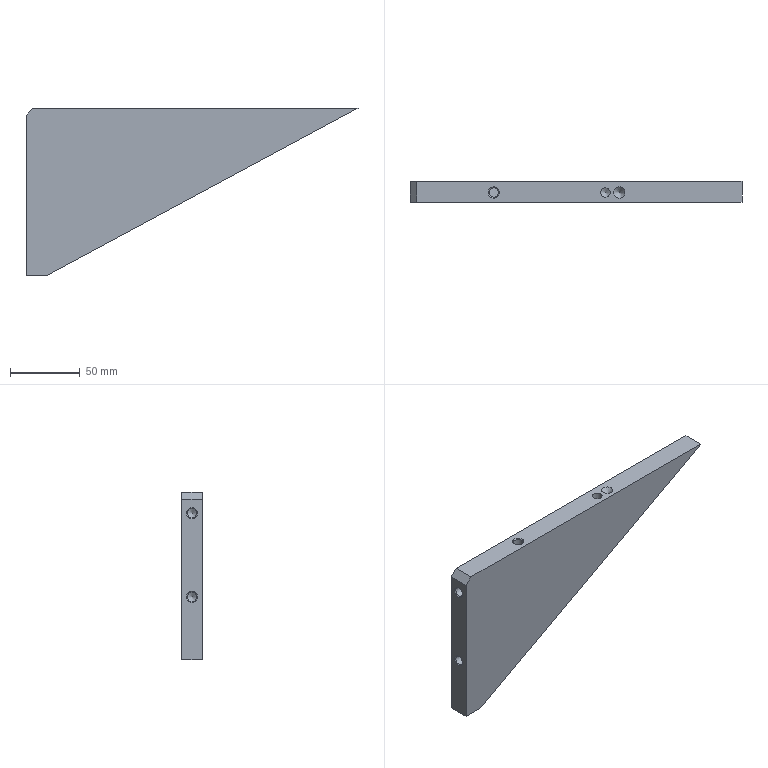Part | STEP file | 冲床-300配套压波_id978_x_t | 1 solid | 19 faces | box 237.857 x 15 x 120 mm | volume 223740 mm3 | cone 8 | plane 7 | cylinder 4 | commonest cylinder face diameters 6.8 x4
STEP:
#1=CARTESIAN_POINT('',(1960.,75.,-230.));
#2=VERTEX_POINT('',#1);
#3=CARTESIAN_POINT('',(2192.857,75.,-230.));
#4=VERTEX_POINT('',#3);
#5=CARTESIAN_POINT('',(2165.,75.,-230.));
#6=DIRECTION('',(1.,0.,0.));
#7=VECTOR('',#6,1.);
#8=LINE('',#5,#7);
#9=EDGE_CURVE('',#2,#4,#8,.T.);
#10=ORIENTED_EDGE('',*,*,#9,.F.);
#11=CARTESIAN_POINT('',(1955.,75.,-235.));
#12=VERTEX_POINT('',#11);
#13=CARTESIAN_POINT('',(1967.5,75.,-222.5));
#14=DIRECTION('',(-0.7071,0.,-0.7071));
#15=VECTOR('',#14,1.);
#16=LINE('',#13,#15);
#17=EDGE_CURVE('',#2,#12,#16,.T.);
#18=ORIENTED_EDGE('',*,*,#17,.T.);
#19=CARTESIAN_POINT('',(1955.,75.,-350.));
#20=VERTEX_POINT('',#19);
#21=CARTESIAN_POINT('',(1955.,75.,-230.));
#22=DIRECTION('',(0.,0.,1.));
#23=VECTOR('',#22,1.);
#24=LINE('',#21,#23);
#25=EDGE_CURVE('',#20,#12,#24,.T.);
#26=ORIENTED_EDGE('',*,*,#25,.F.);
#27=CARTESIAN_POINT('',(1970.,75.,-350.));
#28=VERTEX_POINT('',#27);
#29=CARTESIAN_POINT('',(1955.,75.,-350.));
#30=DIRECTION('',(-1.,0.,0.));
#31=VECTOR('',#30,1.);
#32=LINE('',#29,#31);
#33=EDGE_CURVE('',#28,#20,#32,.T.);
#34=ORIENTED_EDGE('',*,*,#33,.F.);
#35=CARTESIAN_POINT('',(1970.,75.,-350.));
#36=DIRECTION('',(-0.8805,0.,-0.4741));
#37=VECTOR('',#36,1.);
#38=LINE('',#35,#37);
#39=EDGE_CURVE('',#4,#28,#38,.T.);
#40=ORIENTED_EDGE('',*,*,#39,.F.);
#41=EDGE_LOOP('',(#10,#18,#26,#34,#40));
#42=FACE_OUTER_BOUND('',#41,.T.);
#43=CARTESIAN_POINT('',(2135.,75.,-390.));
#44=DIRECTION('',(0.,1.,0.));
#45=DIRECTION('',(0.,0.,-1.));
#46=AXIS2_PLACEMENT_3D('',#43,#44,#45);
#47=PLANE('',#46);
#48=ADVANCED_FACE('',(#42),#47,.F.);
#49=CARTESIAN_POINT('',(1955.,90.,-350.));
#50=VERTEX_POINT('',#49);
#51=CARTESIAN_POINT('',(1955.,-58.5,-350.));
#52=DIRECTION('',(0.,-1.,0.));
#53=VECTOR('',#52,1.);
#54=LINE('',#51,#53);
#55=EDGE_CURVE('',#50,#20,#54,.T.);
#56=ORIENTED_EDGE('',*,*,#55,.F.);
#57=CARTESIAN_POINT('',(1970.,90.,-350.));
#58=VERTEX_POINT('',#57);
#59=CARTESIAN_POINT('',(1955.,90.,-350.));
#60=DIRECTION('',(-1.,0.,0.));
#61=VECTOR('',#60,1.);
#62=LINE('',#59,#61);
#63=EDGE_CURVE('',#58,#50,#62,.T.);
#64=ORIENTED_EDGE('',*,*,#63,.F.);
#65=CARTESIAN_POINT('',(1970.,-58.5,-350.));
#66=DIRECTION('',(0.,-1.,0.));
#67=VECTOR('',#66,1.);
#68=LINE('',#65,#67);
#69=EDGE_CURVE('',#58,#28,#68,.T.);
#70=ORIENTED_EDGE('',*,*,#69,.T.);
#71=ORIENTED_EDGE('',*,*,#33,.T.);
#72=EDGE_LOOP('',(#56,#64,#70,#71));
#73=FACE_OUTER_BOUND('',#72,.T.);
#74=CARTESIAN_POINT('',(1955.,-58.5,-350.));
#75=DIRECTION('',(0.,0.,-1.));
#76=DIRECTION('',(-1.,0.,0.));
#77=AXIS2_PLACEMENT_3D('',#74,#75,#76);
#78=PLANE('',#77);
#79=ADVANCED_FACE('',(#73),#78,.T.);
#80=ORIENTED_EDGE('',*,*,#69,.F.);
#81=CARTESIAN_POINT('',(2192.857,90.,-230.));
#82=VERTEX_POINT('',#81);
#83=CARTESIAN_POINT('',(1970.,90.,-350.));
#84=DIRECTION('',(-0.8805,0.,-0.4741));
#85=VECTOR('',#84,1.);
#86=LINE('',#83,#85);
#87=EDGE_CURVE('',#82,#58,#86,.T.);
#88=ORIENTED_EDGE('',*,*,#87,.F.);
#89=CARTESIAN_POINT('',(2192.857,-58.5,-230.));
#90=DIRECTION('',(0.,1.,0.));
#91=VECTOR('',#90,1.);
#92=LINE('',#89,#91);
#93=EDGE_CURVE('',#4,#82,#92,.T.);
#94=ORIENTED_EDGE('',*,*,#93,.F.);
#95=ORIENTED_EDGE('',*,*,#39,.T.);
#96=EDGE_LOOP('',(#80,#88,#94,#95));
#97=FACE_OUTER_BOUND('',#96,.T.);
#98=CARTESIAN_POINT('',(1970.,-58.5,-350.));
#99=DIRECTION('',(0.4741,0.,-0.8805));
#100=DIRECTION('',(-0.8805,0.,-0.4741));
#101=AXIS2_PLACEMENT_3D('',#98,#99,#100);
#102=PLANE('',#101);
#103=ADVANCED_FACE('',(#97),#102,.T.);
#104=CARTESIAN_POINT('',(1955.,90.,-235.));
#105=VERTEX_POINT('',#104);
#106=CARTESIAN_POINT('',(1955.,90.,-230.));
#107=DIRECTION('',(0.,0.,1.));
#108=VECTOR('',#107,1.);
#109=LINE('',#106,#108);
#110=EDGE_CURVE('',#50,#105,#109,.T.);
#111=ORIENTED_EDGE('',*,*,#110,.T.);
#112=CARTESIAN_POINT('',(1960.,90.,-230.));
#113=VERTEX_POINT('',#112);
#114=CARTESIAN_POINT('',(1960.,90.,-230.));
#115=DIRECTION('',(0.7071,0.,0.7071));
#116=VECTOR('',#115,1.);
#117=LINE('',#114,#116);
#118=EDGE_CURVE('',#105,#113,#117,.T.);
#119=ORIENTED_EDGE('',*,*,#118,.T.);
#120=CARTESIAN_POINT('',(2165.,90.,-230.));
#121=DIRECTION('',(1.,0.,0.));
#122=VECTOR('',#121,1.);
#123=LINE('',#120,#122);
#124=EDGE_CURVE('',#113,#82,#123,.T.);
#125=ORIENTED_EDGE('',*,*,#124,.T.);
#126=ORIENTED_EDGE('',*,*,#87,.T.);
#127=ORIENTED_EDGE('',*,*,#63,.T.);
#128=EDGE_LOOP('',(#111,#119,#125,#126,#127));
#129=FACE_OUTER_BOUND('',#128,.T.);
#130=CARTESIAN_POINT('',(1455.,90.,-90.));
#131=DIRECTION('',(0.,-1.,0.));
#132=DIRECTION('',(0.,0.,1.));
#133=AXIS2_PLACEMENT_3D('',#130,#131,#132);
#134=PLANE('',#133);
#135=ADVANCED_FACE('',(#129),#134,.F.);
#136=CARTESIAN_POINT('',(1955.,82.5,-301.));
#137=VERTEX_POINT('',#136);
#138=CARTESIAN_POINT('',(1955.,82.5,-305.));
#139=DIRECTION('',(1.,0.,0.));
#140=DIRECTION('',(0.,0.,1.));
#141=AXIS2_PLACEMENT_3D('',#138,#139,#140);
#142=CIRCLE('',#141,4.);
#143=EDGE_CURVE('',#137,#137,#142,.T.);
#144=ORIENTED_EDGE('',*,*,#143,.T.);
#145=EDGE_LOOP('',(#144));
#146=FACE_BOUND('',#145,.T.);
#147=CARTESIAN_POINT('',(1955.,82.5,-241.));
#148=VERTEX_POINT('',#147);
#149=CARTESIAN_POINT('',(1955.,82.5,-245.));
#150=DIRECTION('',(1.,0.,0.));
#151=DIRECTION('',(0.,0.,1.));
#152=AXIS2_PLACEMENT_3D('',#149,#150,#151);
#153=CIRCLE('',#152,4.);
#154=EDGE_CURVE('',#148,#148,#153,.T.);
#155=ORIENTED_EDGE('',*,*,#154,.T.);
#156=EDGE_LOOP('',(#155));
#157=FACE_BOUND('',#156,.T.);
#158=ORIENTED_EDGE('',*,*,#25,.T.);
#159=CARTESIAN_POINT('',(1955.,-58.5,-235.));
#160=DIRECTION('',(0.,1.,0.));
#161=VECTOR('',#160,1.);
#162=LINE('',#159,#161);
#163=EDGE_CURVE('',#12,#105,#162,.T.);
#164=ORIENTED_EDGE('',*,*,#163,.T.);
#165=ORIENTED_EDGE('',*,*,#110,.F.);
#166=ORIENTED_EDGE('',*,*,#55,.T.);
#167=EDGE_LOOP('',(#158,#164,#165,#166));
#168=FACE_BOUND('',#167,.T.);
#169=CARTESIAN_POINT('',(1955.,-58.5,-230.));
#170=DIRECTION('',(-1.,0.,0.));
#171=DIRECTION('',(0.,0.,1.));
#172=AXIS2_PLACEMENT_3D('',#169,#170,#171);
#173=PLANE('',#172);
#174=ADVANCED_FACE('',(#146,#157,#168),#173,.T.);
#175=CARTESIAN_POINT('',(2098.4,82.01,-230.));
#176=VERTEX_POINT('',#175);
#177=CARTESIAN_POINT('',(2095.,82.01,-230.));
#178=DIRECTION('',(0.,0.,1.));
#179=DIRECTION('',(1.,0.,0.));
#180=AXIS2_PLACEMENT_3D('',#177,#178,#179);
#181=CIRCLE('',#180,3.4);
#182=EDGE_CURVE('',#176,#176,#181,.T.);
#183=ORIENTED_EDGE('',*,*,#182,.F.);
#184=EDGE_LOOP('',(#183));
#185=FACE_BOUND('',#184,.T.);
#186=CARTESIAN_POINT('',(2109.,82.01,-230.));
#187=VERTEX_POINT('',#186);
#188=CARTESIAN_POINT('',(2105.,82.01,-230.));
#189=DIRECTION('',(0.,0.,-1.));
#190=DIRECTION('',(1.,0.,0.));
#191=AXIS2_PLACEMENT_3D('',#188,#189,#190);
#192=CIRCLE('',#191,4.);
#193=EDGE_CURVE('',#187,#187,#192,.T.);
#194=ORIENTED_EDGE('',*,*,#193,.T.);
#195=EDGE_LOOP('',(#194));
#196=FACE_BOUND('',#195,.T.);
#197=CARTESIAN_POINT('',(2019.,82.01,-230.));
#198=VERTEX_POINT('',#197);
#199=CARTESIAN_POINT('',(2015.,82.01,-230.));
#200=DIRECTION('',(0.,0.,-1.));
#201=DIRECTION('',(1.,0.,0.));
#202=AXIS2_PLACEMENT_3D('',#199,#200,#201);
#203=CIRCLE('',#202,4.);
#204=EDGE_CURVE('',#198,#198,#203,.T.);
#205=ORIENTED_EDGE('',*,*,#204,.T.);
#206=EDGE_LOOP('',(#205));
#207=FACE_BOUND('',#206,.T.);
#208=ORIENTED_EDGE('',*,*,#124,.F.);
#209=CARTESIAN_POINT('',(1960.,-58.5,-230.));
#210=DIRECTION('',(0.,-1.,0.));
#211=VECTOR('',#210,1.);
#212=LINE('',#209,#211);
#213=EDGE_CURVE('',#113,#2,#212,.T.);
#214=ORIENTED_EDGE('',*,*,#213,.T.);
#215=ORIENTED_EDGE('',*,*,#9,.T.);
#216=ORIENTED_EDGE('',*,*,#93,.T.);
#217=EDGE_LOOP('',(#208,#214,#215,#216));
#218=FACE_BOUND('',#217,.T.);
#219=CARTESIAN_POINT('',(2165.,-58.5,-230.));
#220=DIRECTION('',(0.,0.,1.));
#221=DIRECTION('',(1.,0.,0.));
#222=AXIS2_PLACEMENT_3D('',#219,#220,#221);
#223=PLANE('',#222);
#224=ADVANCED_FACE('',(#185,#196,#207,#218),#223,.T.);
#225=CARTESIAN_POINT('',(2018.4,82.01,-268.226));
#226=VERTEX_POINT('',#225);
#227=CARTESIAN_POINT('',(2018.4,81.034,-268.226));
#228=CARTESIAN_POINT('',(2018.4,82.987,-268.226));
#229=CARTESIAN_POINT('',(2017.968,83.879,-267.863));
#230=CARTESIAN_POINT('',(2016.722,85.066,-266.967));
#231=CARTESIAN_POINT('',(2015.925,85.388,-266.449));
#232=CARTESIAN_POINT('',(2014.246,85.43,-265.47));
#233=CARTESIAN_POINT('',(2013.393,85.141,-265.022));
#234=CARTESIAN_POINT('',(2012.046,83.924,-264.347));
#235=CARTESIAN_POINT('',(2011.603,82.987,-264.142));
#236=CARTESIAN_POINT('',(2011.597,81.057,-264.138));
#237=CARTESIAN_POINT('',(2012.032,80.116,-264.34));
#238=CARTESIAN_POINT('',(2013.382,78.884,-265.016));
#239=CARTESIAN_POINT('',(2014.251,78.591,-265.473));
#240=CARTESIAN_POINT('',(2015.915,78.632,-266.443));
#241=CARTESIAN_POINT('',(2016.726,78.96,-266.97));
#242=CARTESIAN_POINT('',(2017.96,80.134,-267.857));
#243=CARTESIAN_POINT('',(2018.4,81.034,-268.226));
#244=CARTESIAN_POINT('',(2018.4,82.987,-268.226));
#245=B_SPLINE_CURVE_WITH_KNOTS('',3,(#227,#228,#229,#230,#231,#232,#233,#234,#235,#236,#237,#238,#239,#240,#241,#242,#243,#244),.UNSPECIFIED.,.T.,.F.,(2,2,2,2,2,2,2,2,2,2,2),(-0.125,0.,0.125,0.25,0.375,0.5,0.625,0.75,0.875,1.,1.125),.UNSPECIFIED.);
#246=EDGE_CURVE('',#226,#226,#245,.T.);
#247=ORIENTED_EDGE('',*,*,#246,.T.);
#248=EDGE_LOOP('',(#247));
#249=FACE_OUTER_BOUND('',#248,.T.);
#250=CARTESIAN_POINT('',(2027.5,82.01,-271.651));
#251=DIRECTION('',(0.,0.,1.));
#252=DIRECTION('',(1.,0.,0.));
#253=AXIS2_PLACEMENT_3D('',#250,#251,#252);
#254=CONICAL_SURFACE('',#253,3.4,59.);
#255=ADVANCED_FACE('',(#249),#254,.F.);
#256=CARTESIAN_POINT('',(2018.4,82.01,-230.6));
#257=VERTEX_POINT('',#256);
#258=CARTESIAN_POINT('',(2015.,82.01,-230.6));
#259=DIRECTION('',(0.,0.,1.));
#260=DIRECTION('',(1.,0.,0.));
#261=AXIS2_PLACEMENT_3D('',#258,#259,#260);
#262=CIRCLE('',#261,3.4);
#263=EDGE_CURVE('',#257,#257,#262,.T.);
#264=ORIENTED_EDGE('',*,*,#263,.T.);
#265=EDGE_LOOP('',(#264));
#266=FACE_BOUND('',#265,.T.);
#267=ORIENTED_EDGE('',*,*,#246,.F.);
#268=EDGE_LOOP('',(#267));
#269=FACE_BOUND('',#268,.T.);
#270=CARTESIAN_POINT('',(2015.,82.01,-230.));
#271=DIRECTION('',(0.,0.,-1.));
#272=DIRECTION('',(-1.,0.,0.));
#273=AXIS2_PLACEMENT_3D('',#270,#271,#272);
#274=CYLINDRICAL_SURFACE('',#273,3.4);
#275=ADVANCED_FACE('',(#266,#269),#274,.F.);
#276=ORIENTED_EDGE('',*,*,#263,.F.);
#277=EDGE_LOOP('',(#276));
#278=FACE_BOUND('',#277,.T.);
#279=ORIENTED_EDGE('',*,*,#204,.F.);
#280=EDGE_LOOP('',(#279));
#281=FACE_BOUND('',#280,.T.);
#282=CARTESIAN_POINT('',(2015.,82.01,-230.));
#283=DIRECTION('',(0.,0.,1.));
#284=DIRECTION('',(1.,0.,0.));
#285=AXIS2_PLACEMENT_3D('',#282,#283,#284);
#286=CONICAL_SURFACE('',#285,4.,45.);
#287=ADVANCED_FACE('',(#278,#281),#286,.F.);
#288=CARTESIAN_POINT('',(2091.6,82.01,-250.));
#289=VERTEX_POINT('',#288);
#290=CARTESIAN_POINT('',(2095.,82.01,-250.));
#291=DIRECTION('',(0.,0.,1.));
#292=DIRECTION('',(-1.,0.,0.));
#293=AXIS2_PLACEMENT_3D('',#290,#291,#292);
#294=CIRCLE('',#293,3.4);
#295=EDGE_CURVE('',#289,#289,#294,.T.);
#296=ORIENTED_EDGE('',*,*,#295,.T.);
#297=EDGE_LOOP('',(#296));
#298=FACE_BOUND('',#297,.T.);
#299=CARTESIAN_POINT('',(2095.,82.01,-252.043));
#300=VERTEX_POINT('',#299);
#301=VERTEX_LOOP('',#300);
#302=FACE_BOUND('',#301,.T.);
#303=CARTESIAN_POINT('',(2095.,82.01,-250.));
#304=DIRECTION('',(0.,0.,1.));
#305=DIRECTION('',(1.,0.,0.));
#306=AXIS2_PLACEMENT_3D('',#303,#304,#305);
#307=CONICAL_SURFACE('',#306,3.4,59.);
#308=ADVANCED_FACE('',(#298,#302),#307,.F.);
#309=ORIENTED_EDGE('',*,*,#182,.T.);
#310=EDGE_LOOP('',(#309));
#311=FACE_BOUND('',#310,.T.);
#312=ORIENTED_EDGE('',*,*,#295,.F.);
#313=EDGE_LOOP('',(#312));
#314=FACE_BOUND('',#313,.T.);
#315=CARTESIAN_POINT('',(2095.,82.01,-230.));
#316=DIRECTION('',(0.,0.,-1.));
#317=DIRECTION('',(-1.,0.,0.));
#318=AXIS2_PLACEMENT_3D('',#315,#316,#317);
#319=CYLINDRICAL_SURFACE('',#318,3.4);
#320=ADVANCED_FACE('',(#311,#314),#319,.F.);
#321=CARTESIAN_POINT('',(2105.,82.01,-234.));
#322=VERTEX_POINT('',#321);
#323=VERTEX_LOOP('',#322);
#324=FACE_BOUND('',#323,.T.);
#325=ORIENTED_EDGE('',*,*,#193,.F.);
#326=EDGE_LOOP('',(#325));
#327=FACE_BOUND('',#326,.T.);
#328=CARTESIAN_POINT('',(2105.,82.01,-230.));
#329=DIRECTION('',(0.,0.,1.));
#330=DIRECTION('',(1.,0.,0.));
#331=AXIS2_PLACEMENT_3D('',#328,#329,#330);
#332=CONICAL_SURFACE('',#331,4.,45.);
#333=ADVANCED_FACE('',(#324,#327),#332,.F.);
#334=CARTESIAN_POINT('',(1975.,82.5,-248.4));
#335=VERTEX_POINT('',#334);
#336=CARTESIAN_POINT('',(1975.,82.5,-245.));
#337=DIRECTION('',(-1.,0.,0.));
#338=DIRECTION('',(0.,0.,-1.));
#339=AXIS2_PLACEMENT_3D('',#336,#337,#338);
#340=CIRCLE('',#339,3.4);
#341=EDGE_CURVE('',#335,#335,#340,.T.);
#342=ORIENTED_EDGE('',*,*,#341,.T.);
#343=EDGE_LOOP('',(#342));
#344=FACE_BOUND('',#343,.T.);
#345=CARTESIAN_POINT('',(1977.043,82.5,-245.));
#346=VERTEX_POINT('',#345);
#347=VERTEX_LOOP('',#346);
#348=FACE_BOUND('',#347,.T.);
#349=CARTESIAN_POINT('',(1975.,82.5,-245.));
#350=DIRECTION('',(-1.,0.,0.));
#351=DIRECTION('',(0.,0.,1.));
#352=AXIS2_PLACEMENT_3D('',#349,#350,#351);
#353=CONICAL_SURFACE('',#352,3.4,59.);
#354=ADVANCED_FACE('',(#344,#348),#353,.F.);
#355=CARTESIAN_POINT('',(1955.6,82.5,-241.6));
#356=VERTEX_POINT('',#355);
#357=CARTESIAN_POINT('',(1955.6,82.5,-245.));
#358=DIRECTION('',(-1.,0.,0.));
#359=DIRECTION('',(0.,0.,1.));
#360=AXIS2_PLACEMENT_3D('',#357,#358,#359);
#361=CIRCLE('',#360,3.4);
#362=EDGE_CURVE('',#356,#356,#361,.T.);
#363=ORIENTED_EDGE('',*,*,#362,.T.);
#364=EDGE_LOOP('',(#363));
#365=FACE_BOUND('',#364,.T.);
#366=ORIENTED_EDGE('',*,*,#341,.F.);
#367=EDGE_LOOP('',(#366));
#368=FACE_BOUND('',#367,.T.);
#369=CARTESIAN_POINT('',(1955.,82.5,-245.));
#370=DIRECTION('',(1.,0.,0.));
#371=DIRECTION('',(0.,0.,-1.));
#372=AXIS2_PLACEMENT_3D('',#369,#370,#371);
#373=CYLINDRICAL_SURFACE('',#372,3.4);
#374=ADVANCED_FACE('',(#365,#368),#373,.F.);
#375=ORIENTED_EDGE('',*,*,#362,.F.);
#376=EDGE_LOOP('',(#375));
#377=FACE_BOUND('',#376,.T.);
#378=ORIENTED_EDGE('',*,*,#154,.F.);
#379=EDGE_LOOP('',(#378));
#380=FACE_BOUND('',#379,.T.);
#381=CARTESIAN_POINT('',(1955.,82.5,-245.));
#382=DIRECTION('',(-1.,0.,0.));
#383=DIRECTION('',(0.,0.,1.));
#384=AXIS2_PLACEMENT_3D('',#381,#382,#383);
#385=CONICAL_SURFACE('',#384,4.,45.);
#386=ADVANCED_FACE('',(#377,#380),#385,.F.);
#387=CARTESIAN_POINT('',(1975.,82.5,-308.4));
#388=VERTEX_POINT('',#387);
#389=CARTESIAN_POINT('',(1975.,82.5,-305.));
#390=DIRECTION('',(-1.,0.,0.));
#391=DIRECTION('',(0.,0.,-1.));
#392=AXIS2_PLACEMENT_3D('',#389,#390,#391);
#393=CIRCLE('',#392,3.4);
#394=EDGE_CURVE('',#388,#388,#393,.T.);
#395=ORIENTED_EDGE('',*,*,#394,.T.);
#396=EDGE_LOOP('',(#395));
#397=FACE_BOUND('',#396,.T.);
#398=CARTESIAN_POINT('',(1977.043,82.5,-305.));
#399=VERTEX_POINT('',#398);
#400=VERTEX_LOOP('',#399);
#401=FACE_BOUND('',#400,.T.);
#402=CARTESIAN_POINT('',(1975.,82.5,-305.));
#403=DIRECTION('',(-1.,0.,0.));
#404=DIRECTION('',(0.,0.,1.));
#405=AXIS2_PLACEMENT_3D('',#402,#403,#404);
#406=CONICAL_SURFACE('',#405,3.4,59.);
#407=ADVANCED_FACE('',(#397,#401),#406,.F.);
#408=CARTESIAN_POINT('',(1955.6,82.5,-301.6));
#409=VERTEX_POINT('',#408);
#410=CARTESIAN_POINT('',(1955.6,82.5,-305.));
#411=DIRECTION('',(-1.,0.,0.));
#412=DIRECTION('',(0.,0.,1.));
#413=AXIS2_PLACEMENT_3D('',#410,#411,#412);
#414=CIRCLE('',#413,3.4);
#415=EDGE_CURVE('',#409,#409,#414,.T.);
#416=ORIENTED_EDGE('',*,*,#415,.T.);
#417=EDGE_LOOP('',(#416));
#418=FACE_BOUND('',#417,.T.);
#419=ORIENTED_EDGE('',*,*,#394,.F.);
#420=EDGE_LOOP('',(#419));
#421=FACE_BOUND('',#420,.T.);
#422=CARTESIAN_POINT('',(1955.,82.5,-305.));
#423=DIRECTION('',(1.,0.,0.));
#424=DIRECTION('',(0.,0.,-1.));
#425=AXIS2_PLACEMENT_3D('',#422,#423,#424);
#426=CYLINDRICAL_SURFACE('',#425,3.4);
#427=ADVANCED_FACE('',(#418,#421),#426,.F.);
#428=ORIENTED_EDGE('',*,*,#415,.F.);
#429=EDGE_LOOP('',(#428));
#430=FACE_BOUND('',#429,.T.);
#431=ORIENTED_EDGE('',*,*,#143,.F.);
#432=EDGE_LOOP('',(#431));
#433=FACE_BOUND('',#432,.T.);
#434=CARTESIAN_POINT('',(1955.,82.5,-305.));
#435=DIRECTION('',(-1.,0.,0.));
#436=DIRECTION('',(0.,0.,1.));
#437=AXIS2_PLACEMENT_3D('',#434,#435,#436);
#438=CONICAL_SURFACE('',#437,4.,45.);
#439=ADVANCED_FACE('',(#430,#433),#438,.F.);
#440=ORIENTED_EDGE('',*,*,#118,.F.);
#441=ORIENTED_EDGE('',*,*,#163,.F.);
#442=ORIENTED_EDGE('',*,*,#17,.F.);
#443=ORIENTED_EDGE('',*,*,#213,.F.);
#444=EDGE_LOOP('',(#440,#441,#442,#443));
#445=FACE_OUTER_BOUND('',#444,.T.);
#446=CARTESIAN_POINT('',(1960.,-58.5,-230.));
#447=DIRECTION('',(0.7071,0.,-0.7071));
#448=DIRECTION('',(0.,-1.,0.));
#449=AXIS2_PLACEMENT_3D('',#446,#447,#448);
#450=PLANE('',#449);
#451=ADVANCED_FACE('',(#445),#450,.F.);
#452=CLOSED_SHELL('',(#48,#79,#103,#135,#174,#224,#255,#275,#287,#308,#320,#333,#354,#374,#386,#407,#427,#439,#451));
#453=MANIFOLD_SOLID_BREP('',#452);
#454=(LENGTH_UNIT()NAMED_UNIT(*)SI_UNIT(.MILLI.,.METRE.));
#455=UNCERTAINTY_MEASURE_WITH_UNIT(LENGTH_MEASURE(0.0508),#454,'','');
#456=(NAMED_UNIT(*)PLANE_ANGLE_UNIT()SI_UNIT($,.RADIAN.));
#457=PLANE_ANGLE_MEASURE_WITH_UNIT(PLANE_ANGLE_MEASURE(0.01745),#456);
#458=DIMENSIONAL_EXPONENTS(0.,0.,0.,0.,0.,0.,0.);
#459=(CONVERSION_BASED_UNIT('DEGREE',#457)NAMED_UNIT(#458)PLANE_ANGLE_UNIT());
#460=(NAMED_UNIT(*)SI_UNIT($,.STERADIAN.)SOLID_ANGLE_UNIT());
#461=(GEOMETRIC_REPRESENTATION_CONTEXT(3)GLOBAL_UNCERTAINTY_ASSIGNED_CONTEXT((#455))GLOBAL_UNIT_ASSIGNED_CONTEXT((#454,#459,#460))REPRESENTATION_CONTEXT('',''));
#462=ADVANCED_BREP_SHAPE_REPRESENTATION('',(#453),#461);